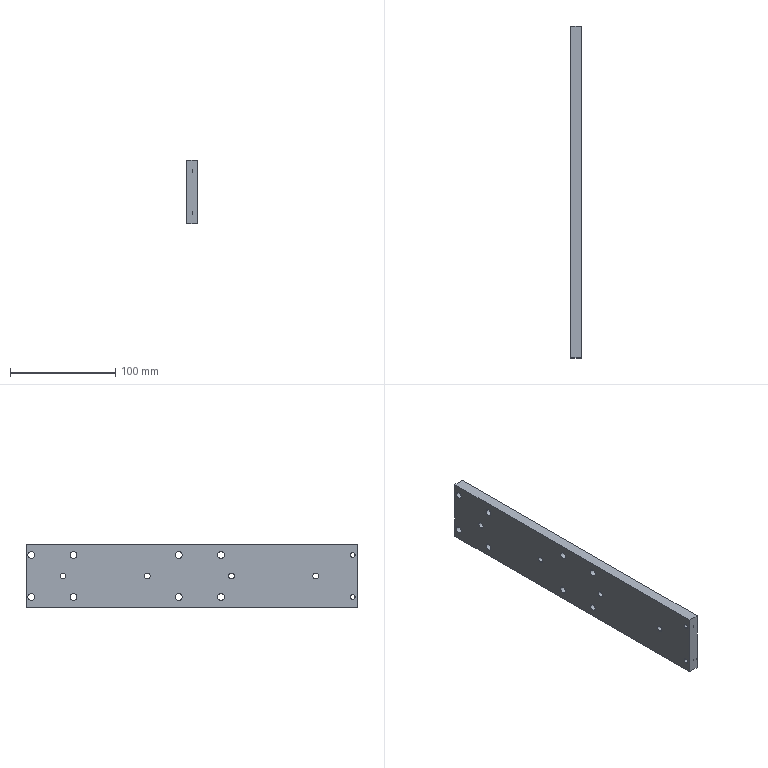Part | STEP file | 09-35 Support plate | 1 solid | 52 faces | box 10 x 315 x 60 mm | volume 183442 mm3 | cylinder 40 | plane 12 | commonest cylinder face diameters 6.5 x16 5.5 x8 10 x8 4.5 x4 9 x4